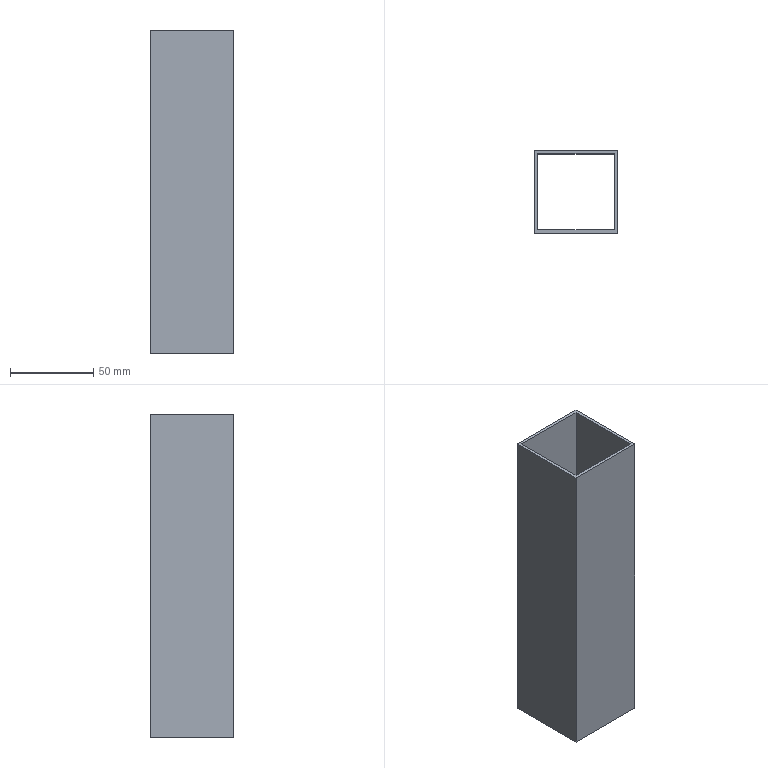Part | SolidWorks | features Extrusion 1, ICE 1 | 1 solid | 10 faces | box 50 x 50 x 194.4 mm | volume 74650 mm3 | plane 10
STEP:
#1=CARTESIAN_POINT('',(25.,-25.,194.4));
#2=VERTEX_POINT('',#1);
#3=CARTESIAN_POINT('',(25.,25.,194.4));
#4=VERTEX_POINT('',#3);
#5=CARTESIAN_POINT('',(25.,-25.,194.4));
#6=DIRECTION('',(0.,1.,0.));
#7=VECTOR('',#6,1000.);
#8=LINE('',#5,#7);
#9=EDGE_CURVE('',#2,#4,#8,.T.);
#10=ORIENTED_EDGE('',*,*,#9,.T.);
#11=CARTESIAN_POINT('',(-25.,25.,194.4));
#12=VERTEX_POINT('',#11);
#13=CARTESIAN_POINT('',(-25.,25.,194.4));
#14=DIRECTION('',(-1.,0.,0.));
#15=VECTOR('',#14,1000.);
#16=LINE('',#13,#15);
#17=EDGE_CURVE('',#4,#12,#16,.T.);
#18=ORIENTED_EDGE('',*,*,#17,.T.);
#19=CARTESIAN_POINT('',(-25.,-25.,194.4));
#20=VERTEX_POINT('',#19);
#21=CARTESIAN_POINT('',(-25.,-25.,194.4));
#22=DIRECTION('',(0.,-1.,0.));
#23=VECTOR('',#22,1000.);
#24=LINE('',#21,#23);
#25=EDGE_CURVE('',#12,#20,#24,.T.);
#26=ORIENTED_EDGE('',*,*,#25,.T.);
#27=CARTESIAN_POINT('',(-25.,-25.,194.4));
#28=DIRECTION('',(1.,0.,0.));
#29=VECTOR('',#28,1000.);
#30=LINE('',#27,#29);
#31=EDGE_CURVE('',#20,#2,#30,.T.);
#32=ORIENTED_EDGE('',*,*,#31,.T.);
#33=EDGE_LOOP('',(#10,#18,#26,#32));
#34=FACE_OUTER_BOUND('',#33,.T.);
#35=CARTESIAN_POINT('',(23.,-23.,194.4));
#36=VERTEX_POINT('',#35);
#37=CARTESIAN_POINT('',(23.,23.,194.4));
#38=VERTEX_POINT('',#37);
#39=CARTESIAN_POINT('',(23.,-23.,194.4));
#40=DIRECTION('',(0.,1.,0.));
#41=VECTOR('',#40,1000.);
#42=LINE('',#39,#41);
#43=EDGE_CURVE('',#36,#38,#42,.T.);
#44=ORIENTED_EDGE('',*,*,#43,.F.);
#45=CARTESIAN_POINT('',(-23.,-23.,194.4));
#46=VERTEX_POINT('',#45);
#47=CARTESIAN_POINT('',(-23.,-23.,194.4));
#48=DIRECTION('',(1.,0.,0.));
#49=VECTOR('',#48,1000.);
#50=LINE('',#47,#49);
#51=EDGE_CURVE('',#46,#36,#50,.T.);
#52=ORIENTED_EDGE('',*,*,#51,.F.);
#53=CARTESIAN_POINT('',(-23.,23.,194.4));
#54=VERTEX_POINT('',#53);
#55=CARTESIAN_POINT('',(-23.,-23.,194.4));
#56=DIRECTION('',(0.,-1.,0.));
#57=VECTOR('',#56,1000.);
#58=LINE('',#55,#57);
#59=EDGE_CURVE('',#54,#46,#58,.T.);
#60=ORIENTED_EDGE('',*,*,#59,.F.);
#61=CARTESIAN_POINT('',(-23.,23.,194.4));
#62=DIRECTION('',(-1.,0.,0.));
#63=VECTOR('',#62,1000.);
#64=LINE('',#61,#63);
#65=EDGE_CURVE('',#38,#54,#64,.T.);
#66=ORIENTED_EDGE('',*,*,#65,.F.);
#67=EDGE_LOOP('',(#44,#52,#60,#66));
#68=FACE_BOUND('',#67,.T.);
#69=CARTESIAN_POINT('',(0.,0.,194.4));
#70=DIRECTION('',(0.,0.,-1.));
#71=DIRECTION('',(-1.,0.,0.));
#72=AXIS2_PLACEMENT_3D('',#69,#70,#71);
#73=PLANE('',#72);
#74=ADVANCED_FACE('',(#34,#68),#73,.F.);
#75=CARTESIAN_POINT('',(25.,-25.,0.));
#76=VERTEX_POINT('',#75);
#77=CARTESIAN_POINT('',(25.,25.,0.));
#78=VERTEX_POINT('',#77);
#79=CARTESIAN_POINT('',(25.,-25.,0.));
#80=DIRECTION('',(0.,1.,0.));
#81=VECTOR('',#80,1000.);
#82=LINE('',#79,#81);
#83=EDGE_CURVE('',#76,#78,#82,.T.);
#84=ORIENTED_EDGE('',*,*,#83,.F.);
#85=CARTESIAN_POINT('',(-25.,-25.,0.));
#86=VERTEX_POINT('',#85);
#87=CARTESIAN_POINT('',(-25.,-25.,0.));
#88=DIRECTION('',(1.,0.,0.));
#89=VECTOR('',#88,1000.);
#90=LINE('',#87,#89);
#91=EDGE_CURVE('',#86,#76,#90,.T.);
#92=ORIENTED_EDGE('',*,*,#91,.F.);
#93=CARTESIAN_POINT('',(-25.,25.,0.));
#94=VERTEX_POINT('',#93);
#95=CARTESIAN_POINT('',(-25.,-25.,0.));
#96=DIRECTION('',(0.,-1.,0.));
#97=VECTOR('',#96,1000.);
#98=LINE('',#95,#97);
#99=EDGE_CURVE('',#94,#86,#98,.T.);
#100=ORIENTED_EDGE('',*,*,#99,.F.);
#101=CARTESIAN_POINT('',(-25.,25.,0.));
#102=DIRECTION('',(-1.,0.,0.));
#103=VECTOR('',#102,1000.);
#104=LINE('',#101,#103);
#105=EDGE_CURVE('',#78,#94,#104,.T.);
#106=ORIENTED_EDGE('',*,*,#105,.F.);
#107=EDGE_LOOP('',(#84,#92,#100,#106));
#108=FACE_OUTER_BOUND('',#107,.T.);
#109=CARTESIAN_POINT('',(-23.,-23.,0.));
#110=VERTEX_POINT('',#109);
#111=CARTESIAN_POINT('',(23.,-23.,0.));
#112=VERTEX_POINT('',#111);
#113=CARTESIAN_POINT('',(-23.,-23.,0.));
#114=DIRECTION('',(1.,0.,0.));
#115=VECTOR('',#114,1000.);
#116=LINE('',#113,#115);
#117=EDGE_CURVE('',#110,#112,#116,.T.);
#118=ORIENTED_EDGE('',*,*,#117,.T.);
#119=CARTESIAN_POINT('',(23.,23.,0.));
#120=VERTEX_POINT('',#119);
#121=CARTESIAN_POINT('',(23.,-23.,0.));
#122=DIRECTION('',(0.,1.,0.));
#123=VECTOR('',#122,1000.);
#124=LINE('',#121,#123);
#125=EDGE_CURVE('',#112,#120,#124,.T.);
#126=ORIENTED_EDGE('',*,*,#125,.T.);
#127=CARTESIAN_POINT('',(-23.,23.,0.));
#128=VERTEX_POINT('',#127);
#129=CARTESIAN_POINT('',(-23.,23.,0.));
#130=DIRECTION('',(-1.,0.,0.));
#131=VECTOR('',#130,1000.);
#132=LINE('',#129,#131);
#133=EDGE_CURVE('',#120,#128,#132,.T.);
#134=ORIENTED_EDGE('',*,*,#133,.T.);
#135=CARTESIAN_POINT('',(-23.,-23.,0.));
#136=DIRECTION('',(0.,-1.,0.));
#137=VECTOR('',#136,1000.);
#138=LINE('',#135,#137);
#139=EDGE_CURVE('',#128,#110,#138,.T.);
#140=ORIENTED_EDGE('',*,*,#139,.T.);
#141=EDGE_LOOP('',(#118,#126,#134,#140));
#142=FACE_BOUND('',#141,.T.);
#143=CARTESIAN_POINT('',(0.,0.,0.));
#144=DIRECTION('',(0.,0.,-1.));
#145=DIRECTION('',(-1.,0.,0.));
#146=AXIS2_PLACEMENT_3D('',#143,#144,#145);
#147=PLANE('',#146);
#148=ADVANCED_FACE('',(#108,#142),#147,.T.);
#149=ORIENTED_EDGE('',*,*,#83,.T.);
#150=CARTESIAN_POINT('',(25.,25.,194.4));
#151=DIRECTION('',(0.,0.,-1.));
#152=VECTOR('',#151,1000.);
#153=LINE('',#150,#152);
#154=EDGE_CURVE('',#4,#78,#153,.T.);
#155=ORIENTED_EDGE('',*,*,#154,.F.);
#156=ORIENTED_EDGE('',*,*,#9,.F.);
#157=CARTESIAN_POINT('',(25.,-25.,194.4));
#158=DIRECTION('',(0.,0.,-1.));
#159=VECTOR('',#158,1000.);
#160=LINE('',#157,#159);
#161=EDGE_CURVE('',#2,#76,#160,.T.);
#162=ORIENTED_EDGE('',*,*,#161,.T.);
#163=EDGE_LOOP('',(#149,#155,#156,#162));
#164=FACE_OUTER_BOUND('',#163,.T.);
#165=CARTESIAN_POINT('',(25.,-25.,194.4));
#166=DIRECTION('',(-1.,0.,0.));
#167=DIRECTION('',(0.,0.,1.));
#168=AXIS2_PLACEMENT_3D('',#165,#166,#167);
#169=PLANE('',#168);
#170=ADVANCED_FACE('',(#164),#169,.F.);
#171=ORIENTED_EDGE('',*,*,#105,.T.);
#172=CARTESIAN_POINT('',(-25.,25.,194.4));
#173=DIRECTION('',(0.,0.,-1.));
#174=VECTOR('',#173,1000.);
#175=LINE('',#172,#174);
#176=EDGE_CURVE('',#12,#94,#175,.T.);
#177=ORIENTED_EDGE('',*,*,#176,.F.);
#178=ORIENTED_EDGE('',*,*,#17,.F.);
#179=ORIENTED_EDGE('',*,*,#154,.T.);
#180=EDGE_LOOP('',(#171,#177,#178,#179));
#181=FACE_OUTER_BOUND('',#180,.T.);
#182=CARTESIAN_POINT('',(-25.,25.,194.4));
#183=DIRECTION('',(0.,-1.,0.));
#184=DIRECTION('',(0.,0.,-1.));
#185=AXIS2_PLACEMENT_3D('',#182,#183,#184);
#186=PLANE('',#185);
#187=ADVANCED_FACE('',(#181),#186,.F.);
#188=ORIENTED_EDGE('',*,*,#99,.T.);
#189=CARTESIAN_POINT('',(-25.,-25.,194.4));
#190=DIRECTION('',(0.,0.,-1.));
#191=VECTOR('',#190,1000.);
#192=LINE('',#189,#191);
#193=EDGE_CURVE('',#20,#86,#192,.T.);
#194=ORIENTED_EDGE('',*,*,#193,.F.);
#195=ORIENTED_EDGE('',*,*,#25,.F.);
#196=ORIENTED_EDGE('',*,*,#176,.T.);
#197=EDGE_LOOP('',(#188,#194,#195,#196));
#198=FACE_OUTER_BOUND('',#197,.T.);
#199=CARTESIAN_POINT('',(-25.,-25.,194.4));
#200=DIRECTION('',(1.,0.,0.));
#201=DIRECTION('',(0.,0.,-1.));
#202=AXIS2_PLACEMENT_3D('',#199,#200,#201);
#203=PLANE('',#202);
#204=ADVANCED_FACE('',(#198),#203,.F.);
#205=ORIENTED_EDGE('',*,*,#91,.T.);
#206=ORIENTED_EDGE('',*,*,#161,.F.);
#207=ORIENTED_EDGE('',*,*,#31,.F.);
#208=ORIENTED_EDGE('',*,*,#193,.T.);
#209=EDGE_LOOP('',(#205,#206,#207,#208));
#210=FACE_OUTER_BOUND('',#209,.T.);
#211=CARTESIAN_POINT('',(-25.,-25.,194.4));
#212=DIRECTION('',(0.,1.,0.));
#213=DIRECTION('',(0.,0.,1.));
#214=AXIS2_PLACEMENT_3D('',#211,#212,#213);
#215=PLANE('',#214);
#216=ADVANCED_FACE('',(#210),#215,.F.);
#217=ORIENTED_EDGE('',*,*,#125,.F.);
#218=CARTESIAN_POINT('',(23.,-23.,194.4));
#219=DIRECTION('',(0.,0.,-1.));
#220=VECTOR('',#219,1000.);
#221=LINE('',#218,#220);
#222=EDGE_CURVE('',#36,#112,#221,.T.);
#223=ORIENTED_EDGE('',*,*,#222,.F.);
#224=ORIENTED_EDGE('',*,*,#43,.T.);
#225=CARTESIAN_POINT('',(23.,23.,194.4));
#226=DIRECTION('',(0.,0.,-1.));
#227=VECTOR('',#226,1000.);
#228=LINE('',#225,#227);
#229=EDGE_CURVE('',#38,#120,#228,.T.);
#230=ORIENTED_EDGE('',*,*,#229,.T.);
#231=EDGE_LOOP('',(#217,#223,#224,#230));
#232=FACE_OUTER_BOUND('',#231,.T.);
#233=CARTESIAN_POINT('',(23.,-23.,194.4));
#234=DIRECTION('',(-1.,0.,0.));
#235=DIRECTION('',(0.,0.,1.));
#236=AXIS2_PLACEMENT_3D('',#233,#234,#235);
#237=PLANE('',#236);
#238=ADVANCED_FACE('',(#232),#237,.T.);
#239=ORIENTED_EDGE('',*,*,#133,.F.);
#240=ORIENTED_EDGE('',*,*,#229,.F.);
#241=ORIENTED_EDGE('',*,*,#65,.T.);
#242=CARTESIAN_POINT('',(-23.,23.,194.4));
#243=DIRECTION('',(0.,0.,-1.));
#244=VECTOR('',#243,1000.);
#245=LINE('',#242,#244);
#246=EDGE_CURVE('',#54,#128,#245,.T.);
#247=ORIENTED_EDGE('',*,*,#246,.T.);
#248=EDGE_LOOP('',(#239,#240,#241,#247));
#249=FACE_OUTER_BOUND('',#248,.T.);
#250=CARTESIAN_POINT('',(-23.,23.,194.4));
#251=DIRECTION('',(0.,-1.,0.));
#252=DIRECTION('',(0.,0.,-1.));
#253=AXIS2_PLACEMENT_3D('',#250,#251,#252);
#254=PLANE('',#253);
#255=ADVANCED_FACE('',(#249),#254,.T.);
#256=ORIENTED_EDGE('',*,*,#139,.F.);
#257=ORIENTED_EDGE('',*,*,#246,.F.);
#258=ORIENTED_EDGE('',*,*,#59,.T.);
#259=CARTESIAN_POINT('',(-23.,-23.,194.4));
#260=DIRECTION('',(0.,0.,-1.));
#261=VECTOR('',#260,1000.);
#262=LINE('',#259,#261);
#263=EDGE_CURVE('',#46,#110,#262,.T.);
#264=ORIENTED_EDGE('',*,*,#263,.T.);
#265=EDGE_LOOP('',(#256,#257,#258,#264));
#266=FACE_OUTER_BOUND('',#265,.T.);
#267=CARTESIAN_POINT('',(-23.,-23.,194.4));
#268=DIRECTION('',(1.,0.,0.));
#269=DIRECTION('',(0.,0.,-1.));
#270=AXIS2_PLACEMENT_3D('',#267,#268,#269);
#271=PLANE('',#270);
#272=ADVANCED_FACE('',(#266),#271,.T.);
#273=ORIENTED_EDGE('',*,*,#117,.F.);
#274=ORIENTED_EDGE('',*,*,#263,.F.);
#275=ORIENTED_EDGE('',*,*,#51,.T.);
#276=ORIENTED_EDGE('',*,*,#222,.T.);
#277=EDGE_LOOP('',(#273,#274,#275,#276));
#278=FACE_OUTER_BOUND('',#277,.T.);
#279=CARTESIAN_POINT('',(-23.,-23.,194.4));
#280=DIRECTION('',(0.,1.,0.));
#281=DIRECTION('',(0.,0.,1.));
#282=AXIS2_PLACEMENT_3D('',#279,#280,#281);
#283=PLANE('',#282);
#284=ADVANCED_FACE('',(#278),#283,.T.);
#285=CLOSED_SHELL('',(#74,#148,#170,#187,#204,#216,#238,#255,#272,#284));
#286=MANIFOLD_SOLID_BREP('',#285);
#287=CARTESIAN_POINT('',(0.,0.,0.));
#288=DIRECTION('',(0.,0.,1.));
#289=DIRECTION('',(1.,0.,0.));
#290=AXIS2_PLACEMENT_3D('',#287,#288,#289);
#291=(LENGTH_UNIT()NAMED_UNIT(*)SI_UNIT(.MILLI.,.METRE.));
#292=UNCERTAINTY_MEASURE_WITH_UNIT(LENGTH_MEASURE(0.00001),#291,'','');
#293=(NAMED_UNIT(*)PLANE_ANGLE_UNIT()SI_UNIT($,.RADIAN.));
#294=(NAMED_UNIT(*)SI_UNIT($,.STERADIAN.)SOLID_ANGLE_UNIT());
#295=(GEOMETRIC_REPRESENTATION_CONTEXT(3)GLOBAL_UNCERTAINTY_ASSIGNED_CONTEXT((#292))GLOBAL_UNIT_ASSIGNED_CONTEXT((#291,#293,#294))REPRESENTATION_CONTEXT('',''));
#296=ADVANCED_BREP_SHAPE_REPRESENTATION('',(#286,#290),#295);